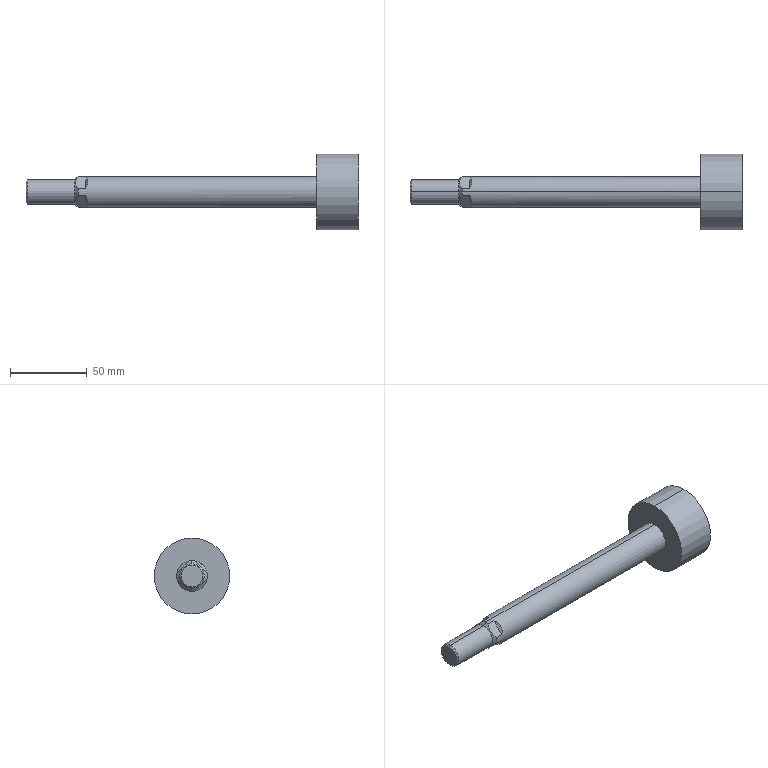Part | SolidWorks | features BaseBody 1 | 1 solid | 21 faces | box 217 x 49.5 x 49.5 mm | volume 107628 mm3 | plane 11 | cylinder 6 | cone 4 | commonest cylinder face diameters 16 x2 20 x2 49.5 x2
STEP:
#1=CARTESIAN_POINT('',(133.,0.,10.));
#2=VERTEX_POINT('',#1);
#3=CARTESIAN_POINT('',(133.,0.,-10.));
#4=VERTEX_POINT('',#3);
#5=CARTESIAN_POINT('',(133.,0.,0.));
#6=DIRECTION('',(-1.,0.,0.));
#7=DIRECTION('',(0.,0.,1.));
#8=AXIS2_PLACEMENT_3D('',#5,#6,#7);
#9=CIRCLE('',#8,10.);
#10=EDGE_CURVE('',#2,#4,#9,.T.);
#11=ORIENTED_EDGE('',*,*,#10,.T.);
#12=CARTESIAN_POINT('',(-23.,0.,-10.));
#13=VERTEX_POINT('',#12);
#14=CARTESIAN_POINT('',(160.,0.,-10.));
#15=DIRECTION('',(-1.,0.,0.));
#16=VECTOR('',#15,1000.);
#17=LINE('',#14,#16);
#18=EDGE_CURVE('',#4,#13,#17,.T.);
#19=ORIENTED_EDGE('',*,*,#18,.T.);
#20=CARTESIAN_POINT('',(-23.,2.285,-9.735));
#21=VERTEX_POINT('',#20);
#22=CARTESIAN_POINT('',(-23.,0.,0.));
#23=DIRECTION('',(1.,0.,0.));
#24=DIRECTION('',(0.,0.,1.));
#25=AXIS2_PLACEMENT_3D('',#22,#23,#24);
#26=CIRCLE('',#25,10.);
#27=EDGE_CURVE('',#13,#21,#26,.T.);
#28=ORIENTED_EDGE('',*,*,#27,.T.);
#29=CARTESIAN_POINT('',(-18.,2.285,-9.735));
#30=VERTEX_POINT('',#29);
#31=CARTESIAN_POINT('',(160.,2.285,-9.735));
#32=DIRECTION('',(1.,0.,0.));
#33=VECTOR('',#32,1000.);
#34=LINE('',#31,#33);
#35=EDGE_CURVE('',#21,#30,#34,.T.);
#36=ORIENTED_EDGE('',*,*,#35,.T.);
#37=CARTESIAN_POINT('',(-18.,9.735,-2.285));
#38=VERTEX_POINT('',#37);
#39=CARTESIAN_POINT('',(-18.,2.285,-9.735));
#40=CARTESIAN_POINT('',(-15.944,6.084,-8.844));
#41=CARTESIAN_POINT('',(-15.944,8.844,-6.084));
#42=CARTESIAN_POINT('',(-18.,9.735,-2.285));
#43=(BOUNDED_CURVE()B_SPLINE_CURVE(3,(#39,#40,#41,#42),.UNSPECIFIED.,.F.,.T.)B_SPLINE_CURVE_WITH_KNOTS((4,4),(2.587,3.696),.UNSPECIFIED.)CURVE()GEOMETRIC_REPRESENTATION_ITEM()RATIONAL_B_SPLINE_CURVE((1.,0.9,0.9,1.))REPRESENTATION_ITEM(''));
#44=EDGE_CURVE('',#30,#38,#43,.T.);
#45=ORIENTED_EDGE('',*,*,#44,.T.);
#46=CARTESIAN_POINT('',(-23.,9.735,-2.285));
#47=VERTEX_POINT('',#46);
#48=CARTESIAN_POINT('',(160.,9.735,-2.285));
#49=DIRECTION('',(-1.,0.,0.));
#50=VECTOR('',#49,1000.);
#51=LINE('',#48,#50);
#52=EDGE_CURVE('',#38,#47,#51,.T.);
#53=ORIENTED_EDGE('',*,*,#52,.T.);
#54=CARTESIAN_POINT('',(-23.,9.735,2.285));
#55=VERTEX_POINT('',#54);
#56=CARTESIAN_POINT('',(-23.,0.,0.));
#57=DIRECTION('',(1.,0.,0.));
#58=DIRECTION('',(0.,0.,1.));
#59=AXIS2_PLACEMENT_3D('',#56,#57,#58);
#60=CIRCLE('',#59,10.);
#61=EDGE_CURVE('',#47,#55,#60,.T.);
#62=ORIENTED_EDGE('',*,*,#61,.T.);
#63=CARTESIAN_POINT('',(-18.,9.735,2.285));
#64=VERTEX_POINT('',#63);
#65=CARTESIAN_POINT('',(160.,9.735,2.285));
#66=DIRECTION('',(1.,0.,0.));
#67=VECTOR('',#66,1000.);
#68=LINE('',#65,#67);
#69=EDGE_CURVE('',#55,#64,#68,.T.);
#70=ORIENTED_EDGE('',*,*,#69,.T.);
#71=CARTESIAN_POINT('',(-18.,2.285,9.735));
#72=VERTEX_POINT('',#71);
#73=CARTESIAN_POINT('',(-18.,9.735,2.285));
#74=CARTESIAN_POINT('',(-15.944,8.844,6.084));
#75=CARTESIAN_POINT('',(-15.944,6.084,8.844));
#76=CARTESIAN_POINT('',(-18.,2.285,9.735));
#77=(BOUNDED_CURVE()B_SPLINE_CURVE(3,(#73,#74,#75,#76),.UNSPECIFIED.,.F.,.F.)B_SPLINE_CURVE_WITH_KNOTS((4,4),(2.587,3.696),.UNSPECIFIED.)CURVE()GEOMETRIC_REPRESENTATION_ITEM()RATIONAL_B_SPLINE_CURVE((1.,0.9,0.9,1.))REPRESENTATION_ITEM(''));
#78=EDGE_CURVE('',#64,#72,#77,.T.);
#79=ORIENTED_EDGE('',*,*,#78,.T.);
#80=CARTESIAN_POINT('',(-23.,2.285,9.735));
#81=VERTEX_POINT('',#80);
#82=CARTESIAN_POINT('',(160.,2.285,9.735));
#83=DIRECTION('',(-1.,0.,0.));
#84=VECTOR('',#83,1000.);
#85=LINE('',#82,#84);
#86=EDGE_CURVE('',#72,#81,#85,.T.);
#87=ORIENTED_EDGE('',*,*,#86,.T.);
#88=CARTESIAN_POINT('',(-23.,0.,10.));
#89=VERTEX_POINT('',#88);
#90=CARTESIAN_POINT('',(-23.,0.,0.));
#91=DIRECTION('',(1.,0.,0.));
#92=DIRECTION('',(0.,0.,1.));
#93=AXIS2_PLACEMENT_3D('',#90,#91,#92);
#94=CIRCLE('',#93,10.);
#95=EDGE_CURVE('',#81,#89,#94,.T.);
#96=ORIENTED_EDGE('',*,*,#95,.T.);
#97=CARTESIAN_POINT('',(160.,0.,10.));
#98=DIRECTION('',(-1.,0.,0.));
#99=VECTOR('',#98,1000.);
#100=LINE('',#97,#99);
#101=EDGE_CURVE('',#2,#89,#100,.T.);
#102=ORIENTED_EDGE('',*,*,#101,.F.);
#103=EDGE_LOOP('',(#11,#19,#28,#36,#45,#53,#62,#70,#79,#87,#96,#102));
#104=FACE_OUTER_BOUND('',#103,.T.);
#105=CARTESIAN_POINT('',(160.,0.,0.));
#106=DIRECTION('',(-1.,0.,0.));
#107=DIRECTION('',(0.,0.,1.));
#108=AXIS2_PLACEMENT_3D('',#105,#106,#107);
#109=CYLINDRICAL_SURFACE('',#108,10.);
#110=ADVANCED_FACE('',(#104),#109,.T.);
#111=CARTESIAN_POINT('',(-25.,0.,-8.));
#112=VERTEX_POINT('',#111);
#113=CARTESIAN_POINT('',(-25.,0.,8.));
#114=VERTEX_POINT('',#113);
#115=CARTESIAN_POINT('',(-25.,0.,0.));
#116=DIRECTION('',(1.,0.,0.));
#117=DIRECTION('',(0.,0.,-1.));
#118=AXIS2_PLACEMENT_3D('',#115,#116,#117);
#119=CIRCLE('',#118,8.);
#120=EDGE_CURVE('',#112,#114,#119,.T.);
#121=ORIENTED_EDGE('',*,*,#120,.T.);
#122=CARTESIAN_POINT('',(-23.,0.,10.));
#123=DIRECTION('',(0.7071,0.,0.7071));
#124=VECTOR('',#123,1000.);
#125=LINE('',#122,#124);
#126=EDGE_CURVE('',#114,#89,#125,.T.);
#127=ORIENTED_EDGE('',*,*,#126,.T.);
#128=ORIENTED_EDGE('',*,*,#95,.F.);
#129=CARTESIAN_POINT('',(-23.,2.285,9.735));
#130=CARTESIAN_POINT('',(-23.432,2.865,9.156));
#131=CARTESIAN_POINT('',(-23.804,3.46,8.561));
#132=CARTESIAN_POINT('',(-24.207,4.392,7.629));
#133=CARTESIAN_POINT('',(-24.315,4.711,7.31));
#134=CARTESIAN_POINT('',(-24.462,5.361,6.66));
#135=CARTESIAN_POINT('',(-24.5,5.685,6.336));
#136=CARTESIAN_POINT('',(-24.5,6.335,5.686));
#137=CARTESIAN_POINT('',(-24.463,6.659,5.362));
#138=CARTESIAN_POINT('',(-24.316,7.308,4.713));
#139=CARTESIAN_POINT('',(-24.208,7.628,4.393));
#140=CARTESIAN_POINT('',(-23.805,8.561,3.46));
#141=CARTESIAN_POINT('',(-23.432,9.156,2.865));
#142=CARTESIAN_POINT('',(-23.,9.735,2.285));
#143=B_SPLINE_CURVE_WITH_KNOTS('',3,(#129,#130,#131,#132,#133,#134,#135,#136,#137,#138,#139,#140,#141,#142),.UNSPECIFIED.,.F.,.F.,(4,2,2,2,2,2,4),(0.,0.002753,0.00413,0.005507,0.006884,0.00826,0.01101),.UNSPECIFIED.);
#144=EDGE_CURVE('',#81,#55,#143,.T.);
#145=ORIENTED_EDGE('',*,*,#144,.T.);
#146=ORIENTED_EDGE('',*,*,#61,.F.);
#147=CARTESIAN_POINT('',(-23.,2.285,-9.735));
#148=CARTESIAN_POINT('',(-23.432,2.865,-9.156));
#149=CARTESIAN_POINT('',(-23.804,3.46,-8.561));
#150=CARTESIAN_POINT('',(-24.207,4.392,-7.629));
#151=CARTESIAN_POINT('',(-24.315,4.711,-7.31));
#152=CARTESIAN_POINT('',(-24.462,5.361,-6.66));
#153=CARTESIAN_POINT('',(-24.5,5.685,-6.336));
#154=CARTESIAN_POINT('',(-24.5,6.335,-5.686));
#155=CARTESIAN_POINT('',(-24.463,6.659,-5.362));
#156=CARTESIAN_POINT('',(-24.316,7.308,-4.713));
#157=CARTESIAN_POINT('',(-24.208,7.628,-4.393));
#158=CARTESIAN_POINT('',(-23.805,8.561,-3.46));
#159=CARTESIAN_POINT('',(-23.432,9.156,-2.865));
#160=CARTESIAN_POINT('',(-23.,9.735,-2.285));
#161=B_SPLINE_CURVE_WITH_KNOTS('',3,(#147,#148,#149,#150,#151,#152,#153,#154,#155,#156,#157,#158,#159,#160),.UNSPECIFIED.,.F.,.F.,(4,2,2,2,2,2,4),(0.,0.002753,0.00413,0.005507,0.006884,0.00826,0.01101),.UNSPECIFIED.);
#162=EDGE_CURVE('',#21,#47,#161,.T.);
#163=ORIENTED_EDGE('',*,*,#162,.F.);
#164=ORIENTED_EDGE('',*,*,#27,.F.);
#165=CARTESIAN_POINT('',(-23.,0.,-10.));
#166=DIRECTION('',(0.7071,0.,-0.7071));
#167=VECTOR('',#166,1000.);
#168=LINE('',#165,#167);
#169=EDGE_CURVE('',#112,#13,#168,.T.);
#170=ORIENTED_EDGE('',*,*,#169,.F.);
#171=EDGE_LOOP('',(#121,#127,#128,#145,#146,#163,#164,#170));
#172=FACE_OUTER_BOUND('',#171,.T.);
#173=CARTESIAN_POINT('',(-23.,0.,0.));
#174=DIRECTION('',(1.,0.,0.));
#175=DIRECTION('',(0.,0.,-1.));
#176=AXIS2_PLACEMENT_3D('',#173,#174,#175);
#177=CONICAL_SURFACE('',#176,10.,0.7854);
#178=ADVANCED_FACE('',(#172),#177,.T.);
#179=ORIENTED_EDGE('',*,*,#120,.F.);
#180=CARTESIAN_POINT('',(-56.08,0.,-8.));
#181=VERTEX_POINT('',#180);
#182=CARTESIAN_POINT('',(160.,0.,-8.));
#183=DIRECTION('',(-1.,0.,0.));
#184=VECTOR('',#183,1000.);
#185=LINE('',#182,#184);
#186=EDGE_CURVE('',#112,#181,#185,.T.);
#187=ORIENTED_EDGE('',*,*,#186,.T.);
#188=CARTESIAN_POINT('',(-56.08,0.,8.));
#189=VERTEX_POINT('',#188);
#190=CARTESIAN_POINT('',(-56.08,0.,0.));
#191=DIRECTION('',(1.,0.,0.));
#192=DIRECTION('',(0.,0.,1.));
#193=AXIS2_PLACEMENT_3D('',#190,#191,#192);
#194=CIRCLE('',#193,8.);
#195=EDGE_CURVE('',#181,#189,#194,.T.);
#196=ORIENTED_EDGE('',*,*,#195,.T.);
#197=CARTESIAN_POINT('',(160.,0.,8.));
#198=DIRECTION('',(-1.,0.,0.));
#199=VECTOR('',#198,1000.);
#200=LINE('',#197,#199);
#201=EDGE_CURVE('',#114,#189,#200,.T.);
#202=ORIENTED_EDGE('',*,*,#201,.F.);
#203=EDGE_LOOP('',(#179,#187,#196,#202));
#204=FACE_OUTER_BOUND('',#203,.T.);
#205=CARTESIAN_POINT('',(160.,0.,0.));
#206=DIRECTION('',(-1.,0.,0.));
#207=DIRECTION('',(0.,0.,1.));
#208=AXIS2_PLACEMENT_3D('',#205,#206,#207);
#209=CYLINDRICAL_SURFACE('',#208,8.);
#210=ADVANCED_FACE('',(#204),#209,.T.);
#211=CARTESIAN_POINT('',(160.,0.,24.75));
#212=VERTEX_POINT('',#211);
#213=CARTESIAN_POINT('',(160.,0.,-24.75));
#214=VERTEX_POINT('',#213);
#215=CARTESIAN_POINT('',(160.,0.,0.));
#216=DIRECTION('',(-1.,0.,0.));
#217=DIRECTION('',(0.,0.,1.));
#218=AXIS2_PLACEMENT_3D('',#215,#216,#217);
#219=CIRCLE('',#218,24.75);
#220=EDGE_CURVE('',#212,#214,#219,.T.);
#221=ORIENTED_EDGE('',*,*,#220,.T.);
#222=CARTESIAN_POINT('',(133.,0.,-24.75));
#223=VERTEX_POINT('',#222);
#224=CARTESIAN_POINT('',(160.,0.,-24.75));
#225=DIRECTION('',(-1.,0.,0.));
#226=VECTOR('',#225,1000.);
#227=LINE('',#224,#226);
#228=EDGE_CURVE('',#214,#223,#227,.T.);
#229=ORIENTED_EDGE('',*,*,#228,.T.);
#230=CARTESIAN_POINT('',(133.,0.,24.75));
#231=VERTEX_POINT('',#230);
#232=CARTESIAN_POINT('',(133.,0.,0.));
#233=DIRECTION('',(1.,0.,0.));
#234=DIRECTION('',(0.,0.,1.));
#235=AXIS2_PLACEMENT_3D('',#232,#233,#234);
#236=CIRCLE('',#235,24.75);
#237=EDGE_CURVE('',#223,#231,#236,.T.);
#238=ORIENTED_EDGE('',*,*,#237,.T.);
#239=CARTESIAN_POINT('',(160.,0.,24.75));
#240=DIRECTION('',(-1.,0.,0.));
#241=VECTOR('',#240,1000.);
#242=LINE('',#239,#241);
#243=EDGE_CURVE('',#212,#231,#242,.T.);
#244=ORIENTED_EDGE('',*,*,#243,.F.);
#245=EDGE_LOOP('',(#221,#229,#238,#244));
#246=FACE_OUTER_BOUND('',#245,.T.);
#247=CARTESIAN_POINT('',(160.,0.,0.));
#248=DIRECTION('',(-1.,0.,0.));
#249=DIRECTION('',(0.,0.,1.));
#250=AXIS2_PLACEMENT_3D('',#247,#248,#249);
#251=CYLINDRICAL_SURFACE('',#250,24.75);
#252=ADVANCED_FACE('',(#246),#251,.T.);
#253=CARTESIAN_POINT('',(-57.,0.,-7.08));
#254=VERTEX_POINT('',#253);
#255=CARTESIAN_POINT('',(-57.,0.,7.08));
#256=VERTEX_POINT('',#255);
#257=CARTESIAN_POINT('',(-57.,0.,0.));
#258=DIRECTION('',(1.,0.,0.));
#259=DIRECTION('',(0.,0.,-1.));
#260=AXIS2_PLACEMENT_3D('',#257,#258,#259);
#261=CIRCLE('',#260,7.08);
#262=EDGE_CURVE('',#254,#256,#261,.T.);
#263=ORIENTED_EDGE('',*,*,#262,.T.);
#264=CARTESIAN_POINT('',(-56.08,0.,8.));
#265=DIRECTION('',(0.7071,0.,0.7071));
#266=VECTOR('',#265,1000.);
#267=LINE('',#264,#266);
#268=EDGE_CURVE('',#256,#189,#267,.T.);
#269=ORIENTED_EDGE('',*,*,#268,.T.);
#270=ORIENTED_EDGE('',*,*,#195,.F.);
#271=CARTESIAN_POINT('',(-56.08,0.,-8.));
#272=DIRECTION('',(0.7071,0.,-0.7071));
#273=VECTOR('',#272,1000.);
#274=LINE('',#271,#273);
#275=EDGE_CURVE('',#254,#181,#274,.T.);
#276=ORIENTED_EDGE('',*,*,#275,.F.);
#277=EDGE_LOOP('',(#263,#269,#270,#276));
#278=FACE_OUTER_BOUND('',#277,.T.);
#279=CARTESIAN_POINT('',(-56.08,0.,0.));
#280=DIRECTION('',(1.,0.,0.));
#281=DIRECTION('',(0.,0.,-1.));
#282=AXIS2_PLACEMENT_3D('',#279,#280,#281);
#283=CONICAL_SURFACE('',#282,8.,0.7854);
#284=ADVANCED_FACE('',(#278),#283,.T.);
#285=ORIENTED_EDGE('',*,*,#18,.F.);
#286=CARTESIAN_POINT('',(133.,0.,0.));
#287=DIRECTION('',(-1.,0.,0.));
#288=DIRECTION('',(0.,0.,1.));
#289=AXIS2_PLACEMENT_3D('',#286,#287,#288);
#290=CIRCLE('',#289,10.);
#291=EDGE_CURVE('',#4,#2,#290,.T.);
#292=ORIENTED_EDGE('',*,*,#291,.T.);
#293=ORIENTED_EDGE('',*,*,#101,.T.);
#294=CARTESIAN_POINT('',(-23.,-2.285,9.735));
#295=VERTEX_POINT('',#294);
#296=CARTESIAN_POINT('',(-23.,0.,0.));
#297=DIRECTION('',(1.,0.,0.));
#298=DIRECTION('',(0.,0.,1.));
#299=AXIS2_PLACEMENT_3D('',#296,#297,#298);
#300=CIRCLE('',#299,10.);
#301=EDGE_CURVE('',#89,#295,#300,.T.);
#302=ORIENTED_EDGE('',*,*,#301,.T.);
#303=CARTESIAN_POINT('',(-18.,-2.285,9.735));
#304=VERTEX_POINT('',#303);
#305=CARTESIAN_POINT('',(160.,-2.285,9.735));
#306=DIRECTION('',(1.,0.,0.));
#307=VECTOR('',#306,1000.);
#308=LINE('',#305,#307);
#309=EDGE_CURVE('',#295,#304,#308,.T.);
#310=ORIENTED_EDGE('',*,*,#309,.T.);
#311=CARTESIAN_POINT('',(-18.,-9.735,2.285));
#312=VERTEX_POINT('',#311);
#313=CARTESIAN_POINT('',(-18.,-2.285,9.735));
#314=CARTESIAN_POINT('',(-15.944,-6.084,8.844));
#315=CARTESIAN_POINT('',(-15.944,-8.844,6.084));
#316=CARTESIAN_POINT('',(-18.,-9.735,2.285));
#317=(BOUNDED_CURVE()B_SPLINE_CURVE(3,(#313,#314,#315,#316),.UNSPECIFIED.,.F.,.T.)B_SPLINE_CURVE_WITH_KNOTS((4,4),(2.587,3.696),.UNSPECIFIED.)CURVE()GEOMETRIC_REPRESENTATION_ITEM()RATIONAL_B_SPLINE_CURVE((1.,0.9,0.9,1.))REPRESENTATION_ITEM(''));
#318=EDGE_CURVE('',#304,#312,#317,.T.);
#319=ORIENTED_EDGE('',*,*,#318,.T.);
#320=CARTESIAN_POINT('',(-23.,-9.735,2.285));
#321=VERTEX_POINT('',#320);
#322=CARTESIAN_POINT('',(160.,-9.735,2.285));
#323=DIRECTION('',(-1.,0.,0.));
#324=VECTOR('',#323,1000.);
#325=LINE('',#322,#324);
#326=EDGE_CURVE('',#312,#321,#325,.T.);
#327=ORIENTED_EDGE('',*,*,#326,.T.);
#328=CARTESIAN_POINT('',(-23.,-9.735,-2.285));
#329=VERTEX_POINT('',#328);
#330=CARTESIAN_POINT('',(-23.,0.,0.));
#331=DIRECTION('',(1.,0.,0.));
#332=DIRECTION('',(0.,0.,1.));
#333=AXIS2_PLACEMENT_3D('',#330,#331,#332);
#334=CIRCLE('',#333,10.);
#335=EDGE_CURVE('',#321,#329,#334,.T.);
#336=ORIENTED_EDGE('',*,*,#335,.T.);
#337=CARTESIAN_POINT('',(-18.,-9.735,-2.285));
#338=VERTEX_POINT('',#337);
#339=CARTESIAN_POINT('',(160.,-9.735,-2.285));
#340=DIRECTION('',(1.,0.,0.));
#341=VECTOR('',#340,1000.);
#342=LINE('',#339,#341);
#343=EDGE_CURVE('',#329,#338,#342,.T.);
#344=ORIENTED_EDGE('',*,*,#343,.T.);
#345=CARTESIAN_POINT('',(-18.,-2.285,-9.735));
#346=VERTEX_POINT('',#345);
#347=CARTESIAN_POINT('',(-18.,-9.735,-2.285));
#348=CARTESIAN_POINT('',(-15.944,-8.844,-6.084));
#349=CARTESIAN_POINT('',(-15.944,-6.084,-8.844));
#350=CARTESIAN_POINT('',(-18.,-2.285,-9.735));
#351=(BOUNDED_CURVE()B_SPLINE_CURVE(3,(#347,#348,#349,#350),.UNSPECIFIED.,.F.,.T.)B_SPLINE_CURVE_WITH_KNOTS((4,4),(2.587,3.696),.UNSPECIFIED.)CURVE()GEOMETRIC_REPRESENTATION_ITEM()RATIONAL_B_SPLINE_CURVE((1.,0.9,0.9,1.))REPRESENTATION_ITEM(''));
#352=EDGE_CURVE('',#338,#346,#351,.T.);
#353=ORIENTED_EDGE('',*,*,#352,.T.);
#354=CARTESIAN_POINT('',(-23.,-2.285,-9.735));
#355=VERTEX_POINT('',#354);
#356=CARTESIAN_POINT('',(160.,-2.285,-9.735));
#357=DIRECTION('',(-1.,0.,0.));
#358=VECTOR('',#357,1000.);
#359=LINE('',#356,#358);
#360=EDGE_CURVE('',#346,#355,#359,.T.);
#361=ORIENTED_EDGE('',*,*,#360,.T.);
#362=CARTESIAN_POINT('',(-23.,0.,0.));
#363=DIRECTION('',(1.,0.,0.));
#364=DIRECTION('',(0.,0.,1.));
#365=AXIS2_PLACEMENT_3D('',#362,#363,#364);
#366=CIRCLE('',#365,10.);
#367=EDGE_CURVE('',#355,#13,#366,.T.);
#368=ORIENTED_EDGE('',*,*,#367,.T.);
#369=EDGE_LOOP('',(#285,#292,#293,#302,#310,#319,#327,#336,#344,#353,#361,#368));
#370=FACE_OUTER_BOUND('',#369,.T.);
#371=CARTESIAN_POINT('',(160.,0.,0.));
#372=DIRECTION('',(-1.,0.,0.));
#373=DIRECTION('',(0.,0.,1.));
#374=AXIS2_PLACEMENT_3D('',#371,#372,#373);
#375=CYLINDRICAL_SURFACE('',#374,10.);
#376=ADVANCED_FACE('',(#370),#375,.T.);
#377=ORIENTED_EDGE('',*,*,#44,.F.);
#378=CARTESIAN_POINT('',(-18.,2.285,-9.735));
#379=DIRECTION('',(0.,0.7071,0.7071));
#380=VECTOR('',#379,1000.);
#381=LINE('',#378,#380);
#382=EDGE_CURVE('',#30,#38,#381,.T.);
#383=ORIENTED_EDGE('',*,*,#382,.T.);
#384=EDGE_LOOP('',(#377,#383));
#385=FACE_OUTER_BOUND('',#384,.T.);
#386=CARTESIAN_POINT('',(-1.,6.01,-30.052));
#387=DIRECTION('',(-0.7071,0.5,-0.5));
#388=DIRECTION('',(-0.5774,0.,0.8165));
#389=AXIS2_PLACEMENT_3D('',#386,#387,#388);
#390=PLANE('',#389);
#391=ADVANCED_FACE('',(#385),#390,.T.);
#392=ORIENTED_EDGE('',*,*,#35,.F.);
#393=ORIENTED_EDGE('',*,*,#162,.T.);
#394=ORIENTED_EDGE('',*,*,#52,.F.);
#395=ORIENTED_EDGE('',*,*,#382,.F.);
#396=EDGE_LOOP('',(#392,#393,#394,#395));
#397=FACE_OUTER_BOUND('',#396,.T.);
#398=CARTESIAN_POINT('',(-18.,-6.01,-18.031));
#399=DIRECTION('',(0.,0.7071,-0.7071));
#400=DIRECTION('',(0.,0.7071,0.7071));
#401=AXIS2_PLACEMENT_3D('',#398,#399,#400);
#402=PLANE('',#401);
#403=ADVANCED_FACE('',(#397),#402,.T.);
#404=ORIENTED_EDGE('',*,*,#126,.F.);
#405=CARTESIAN_POINT('',(-25.,0.,0.));
#406=DIRECTION('',(1.,0.,0.));
#407=DIRECTION('',(0.,0.,-1.));
#408=AXIS2_PLACEMENT_3D('',#405,#406,#407);
#409=CIRCLE('',#408,8.);
#410=EDGE_CURVE('',#114,#112,#409,.T.);
#411=ORIENTED_EDGE('',*,*,#410,.T.);
#412=ORIENTED_EDGE('',*,*,#169,.T.);
#413=ORIENTED_EDGE('',*,*,#367,.F.);
#414=CARTESIAN_POINT('',(-23.,-2.285,-9.735));
#415=CARTESIAN_POINT('',(-23.432,-2.865,-9.156));
#416=CARTESIAN_POINT('',(-23.804,-3.46,-8.561));
#417=CARTESIAN_POINT('',(-24.207,-4.392,-7.629));
#418=CARTESIAN_POINT('',(-24.315,-4.711,-7.31));
#419=CARTESIAN_POINT('',(-24.462,-5.361,-6.66));
#420=CARTESIAN_POINT('',(-24.5,-5.685,-6.336));
#421=CARTESIAN_POINT('',(-24.5,-6.335,-5.686));
#422=CARTESIAN_POINT('',(-24.463,-6.659,-5.362));
#423=CARTESIAN_POINT('',(-24.316,-7.308,-4.713));
#424=CARTESIAN_POINT('',(-24.208,-7.628,-4.393));
#425=CARTESIAN_POINT('',(-23.805,-8.561,-3.46));
#426=CARTESIAN_POINT('',(-23.432,-9.156,-2.865));
#427=CARTESIAN_POINT('',(-23.,-9.735,-2.285));
#428=B_SPLINE_CURVE_WITH_KNOTS('',3,(#414,#415,#416,#417,#418,#419,#420,#421,#422,#423,#424,#425,#426,#427),.UNSPECIFIED.,.F.,.F.,(4,2,2,2,2,2,4),(0.,0.002753,0.00413,0.005507,0.006884,0.00826,0.01101),.UNSPECIFIED.);
#429=EDGE_CURVE('',#355,#329,#428,.T.);
#430=ORIENTED_EDGE('',*,*,#429,.T.);
#431=ORIENTED_EDGE('',*,*,#335,.F.);
#432=CARTESIAN_POINT('',(-23.,-9.735,2.285));
#433=CARTESIAN_POINT('',(-23.432,-9.156,2.865));
#434=CARTESIAN_POINT('',(-23.804,-8.561,3.46));
#435=CARTESIAN_POINT('',(-24.207,-7.629,4.392));
#436=CARTESIAN_POINT('',(-24.315,-7.31,4.711));
#437=CARTESIAN_POINT('',(-24.462,-6.66,5.361));
#438=CARTESIAN_POINT('',(-24.5,-6.336,5.685));
#439=CARTESIAN_POINT('',(-24.5,-5.686,6.335));
#440=CARTESIAN_POINT('',(-24.463,-5.362,6.659));
#441=CARTESIAN_POINT('',(-24.316,-4.713,7.308));
#442=CARTESIAN_POINT('',(-24.208,-4.393,7.628));
#443=CARTESIAN_POINT('',(-23.805,-3.46,8.561));
#444=CARTESIAN_POINT('',(-23.432,-2.865,9.156));
#445=CARTESIAN_POINT('',(-23.,-2.285,9.735));
#446=B_SPLINE_CURVE_WITH_KNOTS('',3,(#432,#433,#434,#435,#436,#437,#438,#439,#440,#441,#442,#443,#444,#445),.UNSPECIFIED.,.F.,.F.,(4,2,2,2,2,2,4),(0.,0.002753,0.00413,0.005507,0.006884,0.00826,0.01101),.UNSPECIFIED.);
#447=EDGE_CURVE('',#321,#295,#446,.T.);
#448=ORIENTED_EDGE('',*,*,#447,.T.);
#449=ORIENTED_EDGE('',*,*,#301,.F.);
#450=EDGE_LOOP('',(#404,#411,#412,#413,#430,#431,#448,#449));
#451=FACE_OUTER_BOUND('',#450,.T.);
#452=CARTESIAN_POINT('',(-23.,0.,0.));
#453=DIRECTION('',(1.,0.,0.));
#454=DIRECTION('',(0.,0.,-1.));
#455=AXIS2_PLACEMENT_3D('',#452,#453,#454);
#456=CONICAL_SURFACE('',#455,10.,0.7854);
#457=ADVANCED_FACE('',(#451),#456,.T.);
#458=ORIENTED_EDGE('',*,*,#343,.F.);
#459=ORIENTED_EDGE('',*,*,#429,.F.);
#460=ORIENTED_EDGE('',*,*,#360,.F.);
#461=CARTESIAN_POINT('',(-18.,-18.031,6.01));
#462=DIRECTION('',(0.,-0.7071,0.7071));
#463=VECTOR('',#462,1000.);
#464=LINE('',#461,#463);
#465=EDGE_CURVE('',#346,#338,#464,.T.);
#466=ORIENTED_EDGE('',*,*,#465,.T.);
#467=EDGE_LOOP('',(#458,#459,#460,#466));
#468=FACE_OUTER_BOUND('',#467,.T.);
#469=CARTESIAN_POINT('',(-18.,-18.031,6.01));
#470=DIRECTION('',(0.,-0.7071,-0.7071));
#471=DIRECTION('',(0.,0.7071,-0.7071));
#472=AXIS2_PLACEMENT_3D('',#469,#470,#471);
#473=PLANE('',#472);
#474=ADVANCED_FACE('',(#468),#473,.T.);
#475=ORIENTED_EDGE('',*,*,#352,.F.);
#476=ORIENTED_EDGE('',*,*,#465,.F.);
#477=EDGE_LOOP('',(#475,#476));
#478=FACE_OUTER_BOUND('',#477,.T.);
#479=CARTESIAN_POINT('',(-1.,-30.052,-6.01));
#480=DIRECTION('',(-0.7071,-0.5,-0.5));
#481=DIRECTION('',(0.5774,-0.8165,0.));
#482=AXIS2_PLACEMENT_3D('',#479,#480,#481);
#483=PLANE('',#482);
#484=ADVANCED_FACE('',(#478),#483,.T.);
#485=ORIENTED_EDGE('',*,*,#309,.F.);
#486=ORIENTED_EDGE('',*,*,#447,.F.);
#487=ORIENTED_EDGE('',*,*,#326,.F.);
#488=CARTESIAN_POINT('',(-18.,-18.031,-6.01));
#489=DIRECTION('',(0.,0.7071,0.7071));
#490=VECTOR('',#489,1000.);
#491=LINE('',#488,#490);
#492=EDGE_CURVE('',#312,#304,#491,.T.);
#493=ORIENTED_EDGE('',*,*,#492,.T.);
#494=EDGE_LOOP('',(#485,#486,#487,#493));
#495=FACE_OUTER_BOUND('',#494,.T.);
#496=CARTESIAN_POINT('',(-57.,-18.031,-6.01));
#497=DIRECTION('',(0.,-0.7071,0.7071));
#498=DIRECTION('',(0.,-0.7071,-0.7071));
#499=AXIS2_PLACEMENT_3D('',#496,#497,#498);
#500=PLANE('',#499);
#501=ADVANCED_FACE('',(#495),#500,.T.);
#502=ORIENTED_EDGE('',*,*,#318,.F.);
#503=ORIENTED_EDGE('',*,*,#492,.F.);
#504=EDGE_LOOP('',(#502,#503));
#505=FACE_OUTER_BOUND('',#504,.T.);
#506=CARTESIAN_POINT('',(-18.,-18.031,-6.01));
#507=DIRECTION('',(-0.7071,-0.5,0.5));
#508=DIRECTION('',(0.5774,0.,0.8165));
#509=AXIS2_PLACEMENT_3D('',#506,#507,#508);
#510=PLANE('',#509);
#511=ADVANCED_FACE('',(#505),#510,.T.);
#512=ORIENTED_EDGE('',*,*,#69,.F.);
#513=ORIENTED_EDGE('',*,*,#144,.F.);
#514=ORIENTED_EDGE('',*,*,#86,.F.);
#515=CARTESIAN_POINT('',(-18.,-6.01,18.031));
#516=DIRECTION('',(0.,0.7071,-0.7071));
#517=VECTOR('',#516,1000.);
#518=LINE('',#515,#517);
#519=EDGE_CURVE('',#72,#64,#518,.T.);
#520=ORIENTED_EDGE('',*,*,#519,.T.);
#521=EDGE_LOOP('',(#512,#513,#514,#520));
#522=FACE_OUTER_BOUND('',#521,.T.);
#523=CARTESIAN_POINT('',(-57.,-6.01,18.031));
#524=DIRECTION('',(0.,0.7071,0.7071));
#525=DIRECTION('',(0.,-0.7071,0.7071));
#526=AXIS2_PLACEMENT_3D('',#523,#524,#525);
#527=PLANE('',#526);
#528=ADVANCED_FACE('',(#522),#527,.T.);
#529=ORIENTED_EDGE('',*,*,#78,.F.);
#530=ORIENTED_EDGE('',*,*,#519,.F.);
#531=EDGE_LOOP('',(#529,#530));
#532=FACE_OUTER_BOUND('',#531,.T.);
#533=CARTESIAN_POINT('',(-18.,-6.01,18.031));
#534=DIRECTION('',(-0.7071,0.5,0.5));
#535=DIRECTION('',(-0.5774,-0.8165,0.));
#536=AXIS2_PLACEMENT_3D('',#533,#534,#535);
#537=PLANE('',#536);
#538=ADVANCED_FACE('',(#532),#537,.T.);
#539=ORIENTED_EDGE('',*,*,#10,.F.);
#540=ORIENTED_EDGE('',*,*,#291,.F.);
#541=EDGE_LOOP('',(#539,#540));
#542=FACE_BOUND('',#541,.T.);
#543=CARTESIAN_POINT('',(133.,0.,0.));
#544=DIRECTION('',(1.,0.,0.));
#545=DIRECTION('',(0.,0.,1.));
#546=AXIS2_PLACEMENT_3D('',#543,#544,#545);
#547=CIRCLE('',#546,24.75);
#548=EDGE_CURVE('',#231,#223,#547,.T.);
#549=ORIENTED_EDGE('',*,*,#548,.F.);
#550=ORIENTED_EDGE('',*,*,#237,.F.);
#551=EDGE_LOOP('',(#549,#550));
#552=FACE_OUTER_BOUND('',#551,.T.);
#553=CARTESIAN_POINT('',(133.,10.,0.));
#554=DIRECTION('',(1.,0.,0.));
#555=DIRECTION('',(0.,0.,-1.));
#556=AXIS2_PLACEMENT_3D('',#553,#554,#555);
#557=PLANE('',#556);
#558=ADVANCED_FACE('',(#542,#552),#557,.F.);
#559=ORIENTED_EDGE('',*,*,#186,.F.);
#560=ORIENTED_EDGE('',*,*,#410,.F.);
#561=ORIENTED_EDGE('',*,*,#201,.T.);
#562=CARTESIAN_POINT('',(-56.08,0.,0.));
#563=DIRECTION('',(1.,0.,0.));
#564=DIRECTION('',(0.,0.,1.));
#565=AXIS2_PLACEMENT_3D('',#562,#563,#564);
#566=CIRCLE('',#565,8.);
#567=EDGE_CURVE('',#189,#181,#566,.T.);
#568=ORIENTED_EDGE('',*,*,#567,.T.);
#569=EDGE_LOOP('',(#559,#560,#561,#568));
#570=FACE_OUTER_BOUND('',#569,.T.);
#571=CARTESIAN_POINT('',(160.,0.,0.));
#572=DIRECTION('',(-1.,0.,0.));
#573=DIRECTION('',(0.,0.,1.));
#574=AXIS2_PLACEMENT_3D('',#571,#572,#573);
#575=CYLINDRICAL_SURFACE('',#574,8.);
#576=ADVANCED_FACE('',(#570),#575,.T.);
#577=ORIENTED_EDGE('',*,*,#228,.F.);
#578=CARTESIAN_POINT('',(160.,0.,0.));
#579=DIRECTION('',(-1.,0.,0.));
#580=DIRECTION('',(0.,0.,1.));
#581=AXIS2_PLACEMENT_3D('',#578,#579,#580);
#582=CIRCLE('',#581,24.75);
#583=EDGE_CURVE('',#214,#212,#582,.T.);
#584=ORIENTED_EDGE('',*,*,#583,.T.);
#585=ORIENTED_EDGE('',*,*,#243,.T.);
#586=ORIENTED_EDGE('',*,*,#548,.T.);
#587=EDGE_LOOP('',(#577,#584,#585,#586));
#588=FACE_OUTER_BOUND('',#587,.T.);
#589=CARTESIAN_POINT('',(160.,0.,0.));
#590=DIRECTION('',(-1.,0.,0.));
#591=DIRECTION('',(0.,0.,1.));
#592=AXIS2_PLACEMENT_3D('',#589,#590,#591);
#593=CYLINDRICAL_SURFACE('',#592,24.75);
#594=ADVANCED_FACE('',(#588),#593,.T.);
#595=ORIENTED_EDGE('',*,*,#268,.F.);
#596=CARTESIAN_POINT('',(-57.,0.,0.));
#597=DIRECTION('',(1.,0.,0.));
#598=DIRECTION('',(0.,0.,-1.));
#599=AXIS2_PLACEMENT_3D('',#596,#597,#598);
#600=CIRCLE('',#599,7.08);
#601=EDGE_CURVE('',#256,#254,#600,.T.);
#602=ORIENTED_EDGE('',*,*,#601,.T.);
#603=ORIENTED_EDGE('',*,*,#275,.T.);
#604=ORIENTED_EDGE('',*,*,#567,.F.);
#605=EDGE_LOOP('',(#595,#602,#603,#604));
#606=FACE_OUTER_BOUND('',#605,.T.);
#607=CARTESIAN_POINT('',(-56.08,0.,0.));
#608=DIRECTION('',(1.,0.,0.));
#609=DIRECTION('',(0.,0.,-1.));
#610=AXIS2_PLACEMENT_3D('',#607,#608,#609);
#611=CONICAL_SURFACE('',#610,8.,0.7854);
#612=ADVANCED_FACE('',(#606),#611,.T.);
#613=ORIENTED_EDGE('',*,*,#220,.F.);
#614=ORIENTED_EDGE('',*,*,#583,.F.);
#615=EDGE_LOOP('',(#613,#614));
#616=FACE_OUTER_BOUND('',#615,.T.);
#617=CARTESIAN_POINT('',(160.,24.75,0.));
#618=DIRECTION('',(-1.,0.,0.));
#619=DIRECTION('',(0.,0.,1.));
#620=AXIS2_PLACEMENT_3D('',#617,#618,#619);
#621=PLANE('',#620);
#622=ADVANCED_FACE('',(#616),#621,.F.);
#623=ORIENTED_EDGE('',*,*,#262,.F.);
#624=ORIENTED_EDGE('',*,*,#601,.F.);
#625=EDGE_LOOP('',(#623,#624));
#626=FACE_OUTER_BOUND('',#625,.T.);
#627=CARTESIAN_POINT('',(-57.,0.,0.));
#628=DIRECTION('',(1.,0.,0.));
#629=DIRECTION('',(0.,0.,-1.));
#630=AXIS2_PLACEMENT_3D('',#627,#628,#629);
#631=PLANE('',#630);
#632=ADVANCED_FACE('',(#626),#631,.F.);
#633=CLOSED_SHELL('',(#110,#178,#210,#252,#284,#376,#391,#403,#457,#474,#484,#501,#511,#528,#538,#558,#576,#594,#612,#622,#632));
#634=MANIFOLD_SOLID_BREP('',#633);
#635=CARTESIAN_POINT('',(0.,0.,0.));
#636=DIRECTION('',(0.,0.,1.));
#637=DIRECTION('',(1.,0.,0.));
#638=AXIS2_PLACEMENT_3D('',#635,#636,#637);
#639=(LENGTH_UNIT()NAMED_UNIT(*)SI_UNIT(.MILLI.,.METRE.));
#640=UNCERTAINTY_MEASURE_WITH_UNIT(LENGTH_MEASURE(0.00001),#639,'','');
#641=(NAMED_UNIT(*)PLANE_ANGLE_UNIT()SI_UNIT($,.RADIAN.));
#642=(NAMED_UNIT(*)SI_UNIT($,.STERADIAN.)SOLID_ANGLE_UNIT());
#643=(GEOMETRIC_REPRESENTATION_CONTEXT(3)GLOBAL_UNCERTAINTY_ASSIGNED_CONTEXT((#640))GLOBAL_UNIT_ASSIGNED_CONTEXT((#639,#641,#642))REPRESENTATION_CONTEXT('',''));
#644=ADVANCED_BREP_SHAPE_REPRESENTATION('',(#634,#638),#643);